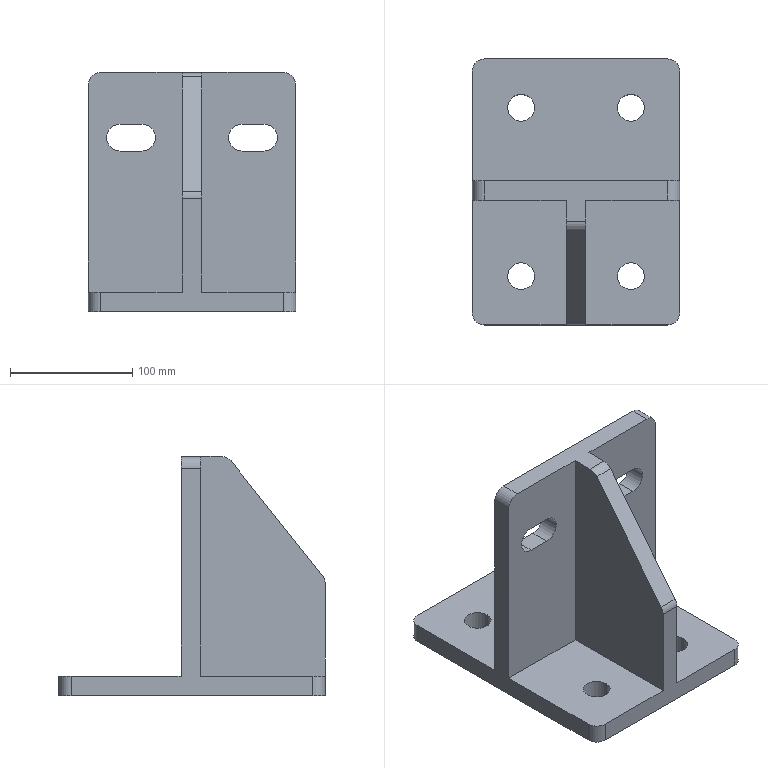Part | STEP file | SX-platform lug | 1 solid | 39 faces | box 170 x 218 x 196 mm | volume 1261021 mm3 | cylinder 20 | plane 19 | commonest cylinder face diameters 22 x12 20 x8